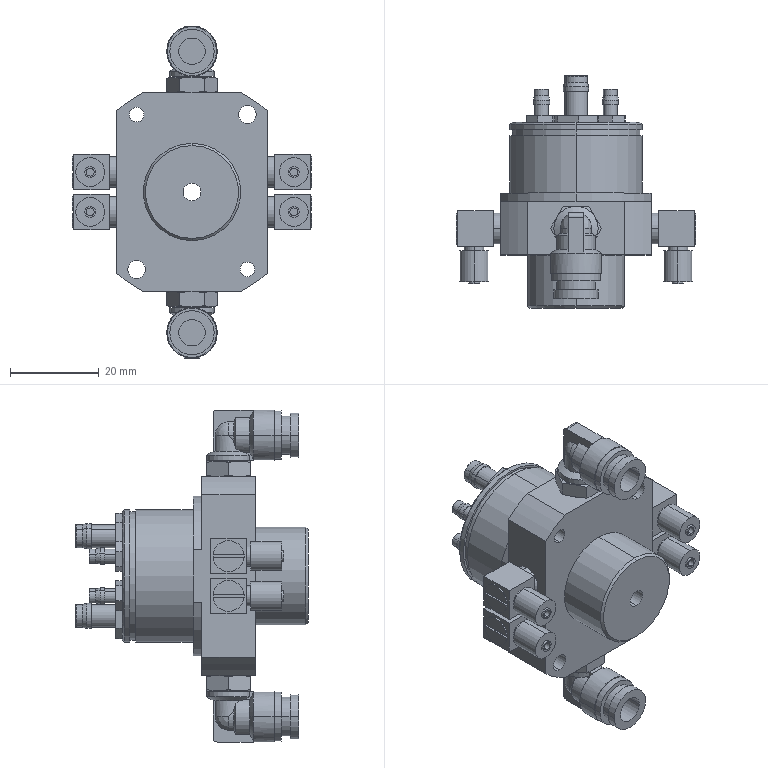Part | SolidWorks | 13 solids | 562 faces | box 54 x 52.5 x 75 mm | volume 38133 mm3 | cylinder 248 | plane 214 | cone 84 | torus 12 | sphere 4 | commonest cylinder face diameters 7 x30 4 x26 2.5 x16 3.2 x16 4.2 x16 5 x16